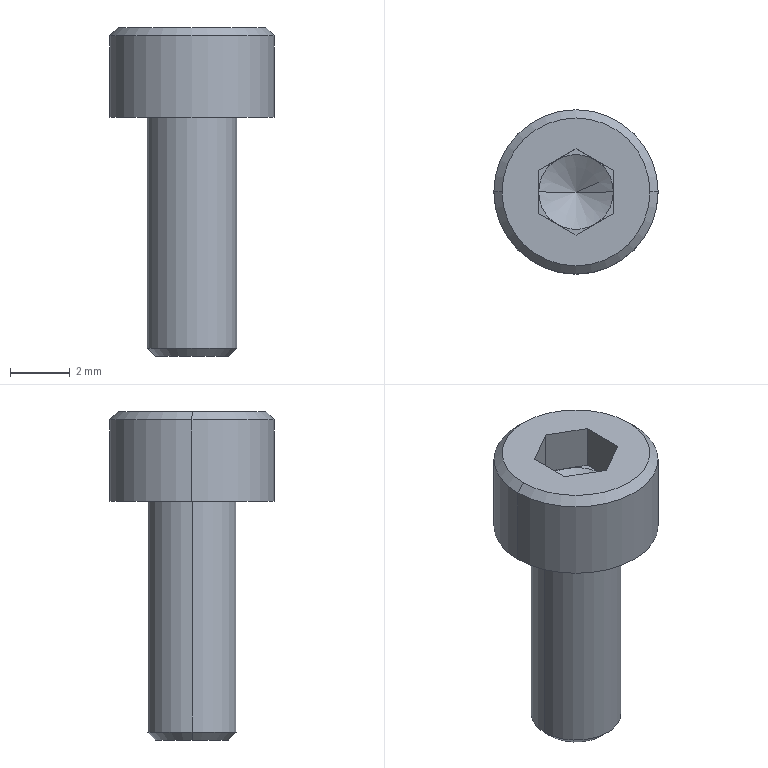Part | SolidWorks | features ICE 2, Chamfer 1, RevCut 1, Revolution 1 | 1 solid | 25 faces | box 5.5 x 5.5 x 11 mm | volume 117.558 mm3 | plane 15 | cone 6 | cylinder 4 | commonest cylinder face diameters 3 x2 5.5 x2
STEP:
#1=CARTESIAN_POINT('',(2.475,0.,3.));
#2=VERTEX_POINT('',#1);
#3=CARTESIAN_POINT('',(-2.475,0.,3.));
#4=VERTEX_POINT('',#3);
#5=CARTESIAN_POINT('',(0.,0.,3.));
#6=DIRECTION('',(0.,0.,1.));
#7=DIRECTION('',(1.,0.,0.));
#8=AXIS2_PLACEMENT_3D('',#5,#6,#7);
#9=CIRCLE('',#8,2.475);
#10=EDGE_CURVE('',#2,#4,#9,.T.);
#11=ORIENTED_EDGE('',*,*,#10,.F.);
#12=CARTESIAN_POINT('',(2.75,0.,2.725));
#13=VERTEX_POINT('',#12);
#14=CARTESIAN_POINT('',(2.475,0.,3.));
#15=DIRECTION('',(0.7071,0.,-0.7071));
#16=VECTOR('',#15,1000.);
#17=LINE('',#14,#16);
#18=EDGE_CURVE('',#2,#13,#17,.T.);
#19=ORIENTED_EDGE('',*,*,#18,.T.);
#20=CARTESIAN_POINT('',(-2.75,0.,2.725));
#21=VERTEX_POINT('',#20);
#22=CARTESIAN_POINT('',(0.,0.,2.725));
#23=DIRECTION('',(0.,0.,-1.));
#24=DIRECTION('',(1.,0.,0.));
#25=AXIS2_PLACEMENT_3D('',#22,#23,#24);
#26=CIRCLE('',#25,2.75);
#27=EDGE_CURVE('',#21,#13,#26,.T.);
#28=ORIENTED_EDGE('',*,*,#27,.F.);
#29=CARTESIAN_POINT('',(-2.475,0.,3.));
#30=DIRECTION('',(-0.7071,0.,-0.7071));
#31=VECTOR('',#30,1000.);
#32=LINE('',#29,#31);
#33=EDGE_CURVE('',#4,#21,#32,.T.);
#34=ORIENTED_EDGE('',*,*,#33,.F.);
#35=EDGE_LOOP('',(#11,#19,#28,#34));
#36=FACE_OUTER_BOUND('',#35,.T.);
#37=CARTESIAN_POINT('',(0.,0.,3.));
#38=DIRECTION('',(0.,0.,-1.));
#39=DIRECTION('',(-1.,0.,0.));
#40=AXIS2_PLACEMENT_3D('',#37,#38,#39);
#41=CONICAL_SURFACE('',#40,2.475,0.7854);
#42=ADVANCED_FACE('',(#36),#41,.T.);
#43=CARTESIAN_POINT('',(-1.225,0.,-8.));
#44=VERTEX_POINT('',#43);
#45=CARTESIAN_POINT('',(1.225,0.,-8.));
#46=VERTEX_POINT('',#45);
#47=CARTESIAN_POINT('',(0.,0.,-8.));
#48=DIRECTION('',(0.,0.,-1.));
#49=DIRECTION('',(-1.,0.,0.));
#50=AXIS2_PLACEMENT_3D('',#47,#48,#49);
#51=CIRCLE('',#50,1.225);
#52=EDGE_CURVE('',#44,#46,#51,.T.);
#53=ORIENTED_EDGE('',*,*,#52,.F.);
#54=CARTESIAN_POINT('',(-1.5,0.,-7.725));
#55=VERTEX_POINT('',#54);
#56=CARTESIAN_POINT('',(-1.225,0.,-8.));
#57=DIRECTION('',(-0.7071,0.,0.7071));
#58=VECTOR('',#57,1000.);
#59=LINE('',#56,#58);
#60=EDGE_CURVE('',#44,#55,#59,.T.);
#61=ORIENTED_EDGE('',*,*,#60,.T.);
#62=CARTESIAN_POINT('',(1.5,0.,-7.725));
#63=VERTEX_POINT('',#62);
#64=CARTESIAN_POINT('',(0.,0.,-7.725));
#65=DIRECTION('',(0.,0.,1.));
#66=DIRECTION('',(-1.,0.,0.));
#67=AXIS2_PLACEMENT_3D('',#64,#65,#66);
#68=CIRCLE('',#67,1.5);
#69=EDGE_CURVE('',#63,#55,#68,.T.);
#70=ORIENTED_EDGE('',*,*,#69,.F.);
#71=CARTESIAN_POINT('',(1.225,0.,-8.));
#72=DIRECTION('',(0.7071,0.,0.7071));
#73=VECTOR('',#72,1000.);
#74=LINE('',#71,#73);
#75=EDGE_CURVE('',#46,#63,#74,.T.);
#76=ORIENTED_EDGE('',*,*,#75,.F.);
#77=EDGE_LOOP('',(#53,#61,#70,#76));
#78=FACE_OUTER_BOUND('',#77,.T.);
#79=CARTESIAN_POINT('',(0.,0.,-8.));
#80=DIRECTION('',(0.,0.,1.));
#81=DIRECTION('',(1.,0.,0.));
#82=AXIS2_PLACEMENT_3D('',#79,#80,#81);
#83=CONICAL_SURFACE('',#82,1.225,0.7854);
#84=ADVANCED_FACE('',(#78),#83,.T.);
#85=CARTESIAN_POINT('',(0.,0.,0.7783));
#86=VERTEX_POINT('',#85);
#87=CARTESIAN_POINT('',(1.25,0.,1.5));
#88=VERTEX_POINT('',#87);
#89=CARTESIAN_POINT('',(0.,0.,0.7783));
#90=DIRECTION('',(0.866,0.,0.5));
#91=VECTOR('',#90,1000.);
#92=LINE('',#89,#91);
#93=EDGE_CURVE('',#86,#88,#92,.T.);
#94=ORIENTED_EDGE('',*,*,#93,.F.);
#95=CARTESIAN_POINT('',(-1.25,0.,1.5));
#96=VERTEX_POINT('',#95);
#97=CARTESIAN_POINT('',(0.,0.,0.7783));
#98=DIRECTION('',(-0.866,0.,0.5));
#99=VECTOR('',#98,1000.);
#100=LINE('',#97,#99);
#101=EDGE_CURVE('',#86,#96,#100,.T.);
#102=ORIENTED_EDGE('',*,*,#101,.T.);
#103=CARTESIAN_POINT('',(-0.625,-1.083,1.5));
#104=VERTEX_POINT('',#103);
#105=CARTESIAN_POINT('',(0.,0.,1.5));
#106=DIRECTION('',(0.,0.,-1.));
#107=DIRECTION('',(-1.,0.,0.));
#108=AXIS2_PLACEMENT_3D('',#105,#106,#107);
#109=CIRCLE('',#108,1.25);
#110=EDGE_CURVE('',#104,#96,#109,.T.);
#111=ORIENTED_EDGE('',*,*,#110,.F.);
#112=CARTESIAN_POINT('',(0.625,-1.083,1.5));
#113=VERTEX_POINT('',#112);
#114=CARTESIAN_POINT('',(0.,0.,1.5));
#115=DIRECTION('',(0.,0.,-1.));
#116=DIRECTION('',(-1.,0.,0.));
#117=AXIS2_PLACEMENT_3D('',#114,#115,#116);
#118=CIRCLE('',#117,1.25);
#119=EDGE_CURVE('',#113,#104,#118,.T.);
#120=ORIENTED_EDGE('',*,*,#119,.F.);
#121=CARTESIAN_POINT('',(0.,0.,1.5));
#122=DIRECTION('',(0.,0.,-1.));
#123=DIRECTION('',(-1.,0.,0.));
#124=AXIS2_PLACEMENT_3D('',#121,#122,#123);
#125=CIRCLE('',#124,1.25);
#126=EDGE_CURVE('',#88,#113,#125,.T.);
#127=ORIENTED_EDGE('',*,*,#126,.F.);
#128=EDGE_LOOP('',(#94,#102,#111,#120,#127));
#129=FACE_OUTER_BOUND('',#128,.T.);
#130=CARTESIAN_POINT('',(0.,0.,1000.778));
#131=DIRECTION('',(0.,0.,1.));
#132=DIRECTION('',(1.,0.,0.));
#133=AXIS2_PLACEMENT_3D('',#130,#131,#132);
#134=CONICAL_SURFACE('',#133,1732.051,1.047);
#135=ADVANCED_FACE('',(#129),#134,.F.);
#136=ORIENTED_EDGE('',*,*,#69,.T.);
#137=CARTESIAN_POINT('',(-1.5,0.,0.));
#138=VERTEX_POINT('',#137);
#139=CARTESIAN_POINT('',(-1.5,0.,-8.));
#140=DIRECTION('',(0.,0.,1.));
#141=VECTOR('',#140,1000.);
#142=LINE('',#139,#141);
#143=EDGE_CURVE('',#55,#138,#142,.T.);
#144=ORIENTED_EDGE('',*,*,#143,.T.);
#145=CARTESIAN_POINT('',(1.5,0.,0.));
#146=VERTEX_POINT('',#145);
#147=CARTESIAN_POINT('',(0.,0.,0.));
#148=DIRECTION('',(0.,0.,-1.));
#149=DIRECTION('',(-1.,0.,0.));
#150=AXIS2_PLACEMENT_3D('',#147,#148,#149);
#151=CIRCLE('',#150,1.5);
#152=EDGE_CURVE('',#138,#146,#151,.T.);
#153=ORIENTED_EDGE('',*,*,#152,.T.);
#154=CARTESIAN_POINT('',(1.5,0.,-8.));
#155=DIRECTION('',(0.,0.,1.));
#156=VECTOR('',#155,1000.);
#157=LINE('',#154,#156);
#158=EDGE_CURVE('',#63,#146,#157,.T.);
#159=ORIENTED_EDGE('',*,*,#158,.F.);
#160=EDGE_LOOP('',(#136,#144,#153,#159));
#161=FACE_OUTER_BOUND('',#160,.T.);
#162=CARTESIAN_POINT('',(0.,0.,-8.));
#163=DIRECTION('',(0.,0.,1.));
#164=DIRECTION('',(1.,0.,0.));
#165=AXIS2_PLACEMENT_3D('',#162,#163,#164);
#166=CYLINDRICAL_SURFACE('',#165,1.5);
#167=ADVANCED_FACE('',(#161),#166,.T.);
#168=CARTESIAN_POINT('',(2.75,0.,0.));
#169=VERTEX_POINT('',#168);
#170=CARTESIAN_POINT('',(-2.75,0.,0.));
#171=VERTEX_POINT('',#170);
#172=CARTESIAN_POINT('',(0.,0.,0.));
#173=DIRECTION('',(0.,0.,1.));
#174=DIRECTION('',(1.,0.,0.));
#175=AXIS2_PLACEMENT_3D('',#172,#173,#174);
#176=CIRCLE('',#175,2.75);
#177=EDGE_CURVE('',#169,#171,#176,.T.);
#178=ORIENTED_EDGE('',*,*,#177,.T.);
#179=CARTESIAN_POINT('',(-2.75,0.,0.));
#180=DIRECTION('',(0.,0.,1.));
#181=VECTOR('',#180,1000.);
#182=LINE('',#179,#181);
#183=EDGE_CURVE('',#171,#21,#182,.T.);
#184=ORIENTED_EDGE('',*,*,#183,.T.);
#185=ORIENTED_EDGE('',*,*,#27,.T.);
#186=CARTESIAN_POINT('',(2.75,0.,0.));
#187=DIRECTION('',(0.,0.,1.));
#188=VECTOR('',#187,1000.);
#189=LINE('',#186,#188);
#190=EDGE_CURVE('',#169,#13,#189,.T.);
#191=ORIENTED_EDGE('',*,*,#190,.F.);
#192=EDGE_LOOP('',(#178,#184,#185,#191));
#193=FACE_OUTER_BOUND('',#192,.T.);
#194=CARTESIAN_POINT('',(0.,0.,0.));
#195=DIRECTION('',(0.,0.,1.));
#196=DIRECTION('',(1.,0.,0.));
#197=AXIS2_PLACEMENT_3D('',#194,#195,#196);
#198=CYLINDRICAL_SURFACE('',#197,2.75);
#199=ADVANCED_FACE('',(#193),#198,.T.);
#200=CARTESIAN_POINT('',(-1.25,0.7217,1.5));
#201=VERTEX_POINT('',#200);
#202=CARTESIAN_POINT('',(-1.25,0.7217,1.5));
#203=DIRECTION('',(0.,-1.,0.));
#204=VECTOR('',#203,1000.);
#205=LINE('',#202,#204);
#206=EDGE_CURVE('',#201,#96,#205,.T.);
#207=ORIENTED_EDGE('',*,*,#206,.T.);
#208=CARTESIAN_POINT('',(-0.625,1.083,1.5));
#209=VERTEX_POINT('',#208);
#210=CARTESIAN_POINT('',(0.,0.,1.5));
#211=DIRECTION('',(0.,0.,-1.));
#212=DIRECTION('',(-1.,0.,0.));
#213=AXIS2_PLACEMENT_3D('',#210,#211,#212);
#214=CIRCLE('',#213,1.25);
#215=EDGE_CURVE('',#96,#209,#214,.T.);
#216=ORIENTED_EDGE('',*,*,#215,.T.);
#217=CARTESIAN_POINT('',(0.,1.443,1.5));
#218=DIRECTION('',(-0.866,-0.5,0.));
#219=VECTOR('',#218,1000.);
#220=LINE('',#217,#219);
#221=EDGE_CURVE('',#209,#201,#220,.T.);
#222=ORIENTED_EDGE('',*,*,#221,.T.);
#223=EDGE_LOOP('',(#207,#216,#222));
#224=FACE_OUTER_BOUND('',#223,.T.);
#225=CARTESIAN_POINT('',(0.,0.,1.5));
#226=DIRECTION('',(0.,0.,1.));
#227=DIRECTION('',(1.,0.,0.));
#228=AXIS2_PLACEMENT_3D('',#225,#226,#227);
#229=PLANE('',#228);
#230=ADVANCED_FACE('',(#224),#229,.T.);
#231=CARTESIAN_POINT('',(0.,1.443,1.5));
#232=VERTEX_POINT('',#231);
#233=CARTESIAN_POINT('',(0.,1.443,1.5));
#234=DIRECTION('',(-0.866,-0.5,0.));
#235=VECTOR('',#234,1000.);
#236=LINE('',#233,#235);
#237=EDGE_CURVE('',#232,#209,#236,.T.);
#238=ORIENTED_EDGE('',*,*,#237,.T.);
#239=CARTESIAN_POINT('',(0.625,1.083,1.5));
#240=VERTEX_POINT('',#239);
#241=CARTESIAN_POINT('',(0.,0.,1.5));
#242=DIRECTION('',(0.,0.,-1.));
#243=DIRECTION('',(-1.,0.,0.));
#244=AXIS2_PLACEMENT_3D('',#241,#242,#243);
#245=CIRCLE('',#244,1.25);
#246=EDGE_CURVE('',#209,#240,#245,.T.);
#247=ORIENTED_EDGE('',*,*,#246,.T.);
#248=CARTESIAN_POINT('',(1.25,0.7217,1.5));
#249=DIRECTION('',(-0.866,0.5,0.));
#250=VECTOR('',#249,1000.);
#251=LINE('',#248,#250);
#252=EDGE_CURVE('',#240,#232,#251,.T.);
#253=ORIENTED_EDGE('',*,*,#252,.T.);
#254=EDGE_LOOP('',(#238,#247,#253));
#255=FACE_OUTER_BOUND('',#254,.T.);
#256=CARTESIAN_POINT('',(0.,0.,1.5));
#257=DIRECTION('',(0.,0.,1.));
#258=DIRECTION('',(1.,0.,0.));
#259=AXIS2_PLACEMENT_3D('',#256,#257,#258);
#260=PLANE('',#259);
#261=ADVANCED_FACE('',(#255),#260,.T.);
#262=CARTESIAN_POINT('',(1.25,0.7217,1.5));
#263=VERTEX_POINT('',#262);
#264=CARTESIAN_POINT('',(1.25,0.7217,1.5));
#265=DIRECTION('',(-0.866,0.5,0.));
#266=VECTOR('',#265,1000.);
#267=LINE('',#264,#266);
#268=EDGE_CURVE('',#263,#240,#267,.T.);
#269=ORIENTED_EDGE('',*,*,#268,.T.);
#270=CARTESIAN_POINT('',(0.,0.,1.5));
#271=DIRECTION('',(0.,0.,-1.));
#272=DIRECTION('',(-1.,0.,0.));
#273=AXIS2_PLACEMENT_3D('',#270,#271,#272);
#274=CIRCLE('',#273,1.25);
#275=EDGE_CURVE('',#240,#88,#274,.T.);
#276=ORIENTED_EDGE('',*,*,#275,.T.);
#277=CARTESIAN_POINT('',(1.25,-0.7217,1.5));
#278=DIRECTION('',(0.,1.,0.));
#279=VECTOR('',#278,1000.);
#280=LINE('',#277,#279);
#281=EDGE_CURVE('',#88,#263,#280,.T.);
#282=ORIENTED_EDGE('',*,*,#281,.T.);
#283=EDGE_LOOP('',(#269,#276,#282));
#284=FACE_OUTER_BOUND('',#283,.T.);
#285=CARTESIAN_POINT('',(0.,0.,1.5));
#286=DIRECTION('',(0.,0.,1.));
#287=DIRECTION('',(1.,0.,0.));
#288=AXIS2_PLACEMENT_3D('',#285,#286,#287);
#289=PLANE('',#288);
#290=ADVANCED_FACE('',(#284),#289,.T.);
#291=CARTESIAN_POINT('',(1.25,-0.7217,1.5));
#292=VERTEX_POINT('',#291);
#293=CARTESIAN_POINT('',(1.25,-0.7217,1.5));
#294=DIRECTION('',(0.,1.,0.));
#295=VECTOR('',#294,1000.);
#296=LINE('',#293,#295);
#297=EDGE_CURVE('',#292,#88,#296,.T.);
#298=ORIENTED_EDGE('',*,*,#297,.T.);
#299=ORIENTED_EDGE('',*,*,#126,.T.);
#300=CARTESIAN_POINT('',(0.,-1.443,1.5));
#301=DIRECTION('',(0.866,0.5,0.));
#302=VECTOR('',#301,1000.);
#303=LINE('',#300,#302);
#304=EDGE_CURVE('',#113,#292,#303,.T.);
#305=ORIENTED_EDGE('',*,*,#304,.T.);
#306=EDGE_LOOP('',(#298,#299,#305));
#307=FACE_OUTER_BOUND('',#306,.T.);
#308=CARTESIAN_POINT('',(0.,0.,1.5));
#309=DIRECTION('',(0.,0.,1.));
#310=DIRECTION('',(1.,0.,0.));
#311=AXIS2_PLACEMENT_3D('',#308,#309,#310);
#312=PLANE('',#311);
#313=ADVANCED_FACE('',(#307),#312,.T.);
#314=CARTESIAN_POINT('',(0.,-1.443,1.5));
#315=VERTEX_POINT('',#314);
#316=CARTESIAN_POINT('',(0.,-1.443,1.5));
#317=DIRECTION('',(0.866,0.5,0.));
#318=VECTOR('',#317,1000.);
#319=LINE('',#316,#318);
#320=EDGE_CURVE('',#315,#113,#319,.T.);
#321=ORIENTED_EDGE('',*,*,#320,.T.);
#322=ORIENTED_EDGE('',*,*,#119,.T.);
#323=CARTESIAN_POINT('',(-1.25,-0.7217,1.5));
#324=DIRECTION('',(0.866,-0.5,0.));
#325=VECTOR('',#324,1000.);
#326=LINE('',#323,#325);
#327=EDGE_CURVE('',#104,#315,#326,.T.);
#328=ORIENTED_EDGE('',*,*,#327,.T.);
#329=EDGE_LOOP('',(#321,#322,#328));
#330=FACE_OUTER_BOUND('',#329,.T.);
#331=CARTESIAN_POINT('',(0.,0.,1.5));
#332=DIRECTION('',(0.,0.,1.));
#333=DIRECTION('',(1.,0.,0.));
#334=AXIS2_PLACEMENT_3D('',#331,#332,#333);
#335=PLANE('',#334);
#336=ADVANCED_FACE('',(#330),#335,.T.);
#337=CARTESIAN_POINT('',(-1.25,-0.7217,1.5));
#338=VERTEX_POINT('',#337);
#339=CARTESIAN_POINT('',(-1.25,-0.7217,1.5));
#340=DIRECTION('',(0.866,-0.5,0.));
#341=VECTOR('',#340,1000.);
#342=LINE('',#339,#341);
#343=EDGE_CURVE('',#338,#104,#342,.T.);
#344=ORIENTED_EDGE('',*,*,#343,.T.);
#345=ORIENTED_EDGE('',*,*,#110,.T.);
#346=CARTESIAN_POINT('',(-1.25,0.7217,1.5));
#347=DIRECTION('',(0.,-1.,0.));
#348=VECTOR('',#347,1000.);
#349=LINE('',#346,#348);
#350=EDGE_CURVE('',#96,#338,#349,.T.);
#351=ORIENTED_EDGE('',*,*,#350,.T.);
#352=EDGE_LOOP('',(#344,#345,#351));
#353=FACE_OUTER_BOUND('',#352,.T.);
#354=CARTESIAN_POINT('',(0.,0.,1.5));
#355=DIRECTION('',(0.,0.,1.));
#356=DIRECTION('',(1.,0.,0.));
#357=AXIS2_PLACEMENT_3D('',#354,#355,#356);
#358=PLANE('',#357);
#359=ADVANCED_FACE('',(#353),#358,.T.);
#360=ORIENTED_EDGE('',*,*,#177,.F.);
#361=CARTESIAN_POINT('',(0.,0.,0.));
#362=DIRECTION('',(0.,0.,1.));
#363=DIRECTION('',(1.,0.,0.));
#364=AXIS2_PLACEMENT_3D('',#361,#362,#363);
#365=CIRCLE('',#364,2.75);
#366=EDGE_CURVE('',#171,#169,#365,.T.);
#367=ORIENTED_EDGE('',*,*,#366,.F.);
#368=EDGE_LOOP('',(#360,#367));
#369=FACE_OUTER_BOUND('',#368,.T.);
#370=CARTESIAN_POINT('',(0.,0.,0.));
#371=DIRECTION('',(0.,0.,-1.));
#372=DIRECTION('',(-1.,0.,0.));
#373=AXIS2_PLACEMENT_3D('',#370,#371,#372);
#374=CIRCLE('',#373,1.5);
#375=EDGE_CURVE('',#146,#138,#374,.T.);
#376=ORIENTED_EDGE('',*,*,#375,.F.);
#377=ORIENTED_EDGE('',*,*,#152,.F.);
#378=EDGE_LOOP('',(#376,#377));
#379=FACE_BOUND('',#378,.T.);
#380=CARTESIAN_POINT('',(2.75,0.,0.));
#381=DIRECTION('',(0.,0.,-1.));
#382=DIRECTION('',(-1.,0.,0.));
#383=AXIS2_PLACEMENT_3D('',#380,#381,#382);
#384=PLANE('',#383);
#385=ADVANCED_FACE('',(#369,#379),#384,.T.);
#386=ORIENTED_EDGE('',*,*,#183,.F.);
#387=ORIENTED_EDGE('',*,*,#366,.T.);
#388=ORIENTED_EDGE('',*,*,#190,.T.);
#389=CARTESIAN_POINT('',(0.,0.,2.725));
#390=DIRECTION('',(0.,0.,-1.));
#391=DIRECTION('',(1.,0.,0.));
#392=AXIS2_PLACEMENT_3D('',#389,#390,#391);
#393=CIRCLE('',#392,2.75);
#394=EDGE_CURVE('',#13,#21,#393,.T.);
#395=ORIENTED_EDGE('',*,*,#394,.T.);
#396=EDGE_LOOP('',(#386,#387,#388,#395));
#397=FACE_OUTER_BOUND('',#396,.T.);
#398=CARTESIAN_POINT('',(0.,0.,0.));
#399=DIRECTION('',(0.,0.,1.));
#400=DIRECTION('',(1.,0.,0.));
#401=AXIS2_PLACEMENT_3D('',#398,#399,#400);
#402=CYLINDRICAL_SURFACE('',#401,2.75);
#403=ADVANCED_FACE('',(#397),#402,.T.);
#404=CARTESIAN_POINT('',(0.,0.,3.));
#405=DIRECTION('',(0.,0.,1.));
#406=DIRECTION('',(1.,0.,0.));
#407=AXIS2_PLACEMENT_3D('',#404,#405,#406);
#408=CIRCLE('',#407,2.475);
#409=EDGE_CURVE('',#4,#2,#408,.T.);
#410=ORIENTED_EDGE('',*,*,#409,.T.);
#411=ORIENTED_EDGE('',*,*,#10,.T.);
#412=EDGE_LOOP('',(#410,#411));
#413=FACE_OUTER_BOUND('',#412,.T.);
#414=CARTESIAN_POINT('',(0.,-1.443,3.));
#415=VERTEX_POINT('',#414);
#416=CARTESIAN_POINT('',(1.25,-0.7217,3.));
#417=VERTEX_POINT('',#416);
#418=CARTESIAN_POINT('',(0.,-1.443,3.));
#419=DIRECTION('',(0.866,0.5,0.));
#420=VECTOR('',#419,1000.);
#421=LINE('',#418,#420);
#422=EDGE_CURVE('',#415,#417,#421,.T.);
#423=ORIENTED_EDGE('',*,*,#422,.F.);
#424=CARTESIAN_POINT('',(-1.25,-0.7217,3.));
#425=VERTEX_POINT('',#424);
#426=CARTESIAN_POINT('',(-1.25,-0.7217,3.));
#427=DIRECTION('',(0.866,-0.5,0.));
#428=VECTOR('',#427,1000.);
#429=LINE('',#426,#428);
#430=EDGE_CURVE('',#425,#415,#429,.T.);
#431=ORIENTED_EDGE('',*,*,#430,.F.);
#432=CARTESIAN_POINT('',(-1.25,0.7217,3.));
#433=VERTEX_POINT('',#432);
#434=CARTESIAN_POINT('',(-1.25,0.7217,3.));
#435=DIRECTION('',(0.,-1.,0.));
#436=VECTOR('',#435,1000.);
#437=LINE('',#434,#436);
#438=EDGE_CURVE('',#433,#425,#437,.T.);
#439=ORIENTED_EDGE('',*,*,#438,.F.);
#440=CARTESIAN_POINT('',(0.,1.443,3.));
#441=VERTEX_POINT('',#440);
#442=CARTESIAN_POINT('',(0.,1.443,3.));
#443=DIRECTION('',(-0.866,-0.5,0.));
#444=VECTOR('',#443,1000.);
#445=LINE('',#442,#444);
#446=EDGE_CURVE('',#441,#433,#445,.T.);
#447=ORIENTED_EDGE('',*,*,#446,.F.);
#448=CARTESIAN_POINT('',(1.25,0.7217,3.));
#449=VERTEX_POINT('',#448);
#450=CARTESIAN_POINT('',(1.25,0.7217,3.));
#451=DIRECTION('',(-0.866,0.5,0.));
#452=VECTOR('',#451,1000.);
#453=LINE('',#450,#452);
#454=EDGE_CURVE('',#449,#441,#453,.T.);
#455=ORIENTED_EDGE('',*,*,#454,.F.);
#456=CARTESIAN_POINT('',(1.25,-0.7217,3.));
#457=DIRECTION('',(0.,1.,0.));
#458=VECTOR('',#457,1000.);
#459=LINE('',#456,#458);
#460=EDGE_CURVE('',#417,#449,#459,.T.);
#461=ORIENTED_EDGE('',*,*,#460,.F.);
#462=EDGE_LOOP('',(#423,#431,#439,#447,#455,#461));
#463=FACE_BOUND('',#462,.T.);
#464=CARTESIAN_POINT('',(0.,0.,3.));
#465=DIRECTION('',(0.,0.,1.));
#466=DIRECTION('',(1.,0.,0.));
#467=AXIS2_PLACEMENT_3D('',#464,#465,#466);
#468=PLANE('',#467);
#469=ADVANCED_FACE('',(#413,#463),#468,.T.);
#470=ORIENTED_EDGE('',*,*,#143,.F.);
#471=CARTESIAN_POINT('',(0.,0.,-7.725));
#472=DIRECTION('',(0.,0.,1.));
#473=DIRECTION('',(-1.,0.,0.));
#474=AXIS2_PLACEMENT_3D('',#471,#472,#473);
#475=CIRCLE('',#474,1.5);
#476=EDGE_CURVE('',#55,#63,#475,.T.);
#477=ORIENTED_EDGE('',*,*,#476,.T.);
#478=ORIENTED_EDGE('',*,*,#158,.T.);
#479=ORIENTED_EDGE('',*,*,#375,.T.);
#480=EDGE_LOOP('',(#470,#477,#478,#479));
#481=FACE_OUTER_BOUND('',#480,.T.);
#482=CARTESIAN_POINT('',(0.,0.,-8.));
#483=DIRECTION('',(0.,0.,1.));
#484=DIRECTION('',(1.,0.,0.));
#485=AXIS2_PLACEMENT_3D('',#482,#483,#484);
#486=CYLINDRICAL_SURFACE('',#485,1.5);
#487=ADVANCED_FACE('',(#481),#486,.T.);
#488=CARTESIAN_POINT('',(0.,0.,-8.));
#489=DIRECTION('',(0.,0.,-1.));
#490=DIRECTION('',(-1.,0.,0.));
#491=AXIS2_PLACEMENT_3D('',#488,#489,#490);
#492=CIRCLE('',#491,1.225);
#493=EDGE_CURVE('',#46,#44,#492,.T.);
#494=ORIENTED_EDGE('',*,*,#493,.T.);
#495=ORIENTED_EDGE('',*,*,#52,.T.);
#496=EDGE_LOOP('',(#494,#495));
#497=FACE_OUTER_BOUND('',#496,.T.);
#498=CARTESIAN_POINT('',(0.,0.,-8.));
#499=DIRECTION('',(0.,0.,-1.));
#500=DIRECTION('',(-1.,0.,0.));
#501=AXIS2_PLACEMENT_3D('',#498,#499,#500);
#502=PLANE('',#501);
#503=ADVANCED_FACE('',(#497),#502,.T.);
#504=ORIENTED_EDGE('',*,*,#422,.T.);
#505=CARTESIAN_POINT('',(1.25,-0.7217,1.5));
#506=DIRECTION('',(0.,0.,1.));
#507=VECTOR('',#506,1000.);
#508=LINE('',#505,#507);
#509=EDGE_CURVE('',#292,#417,#508,.T.);
#510=ORIENTED_EDGE('',*,*,#509,.F.);
#511=ORIENTED_EDGE('',*,*,#304,.F.);
#512=ORIENTED_EDGE('',*,*,#320,.F.);
#513=CARTESIAN_POINT('',(0.,-1.443,1.5));
#514=DIRECTION('',(0.,0.,1.));
#515=VECTOR('',#514,1000.);
#516=LINE('',#513,#515);
#517=EDGE_CURVE('',#315,#415,#516,.T.);
#518=ORIENTED_EDGE('',*,*,#517,.T.);
#519=EDGE_LOOP('',(#504,#510,#511,#512,#518));
#520=FACE_OUTER_BOUND('',#519,.T.);
#521=CARTESIAN_POINT('',(0.,-1.443,1.5));
#522=DIRECTION('',(0.5,-0.866,0.));
#523=DIRECTION('',(0.866,0.5,0.));
#524=AXIS2_PLACEMENT_3D('',#521,#522,#523);
#525=PLANE('',#524);
#526=ADVANCED_FACE('',(#520),#525,.F.);
#527=ORIENTED_EDGE('',*,*,#430,.T.);
#528=ORIENTED_EDGE('',*,*,#517,.F.);
#529=ORIENTED_EDGE('',*,*,#327,.F.);
#530=ORIENTED_EDGE('',*,*,#343,.F.);
#531=CARTESIAN_POINT('',(-1.25,-0.7217,1.5));
#532=DIRECTION('',(0.,0.,1.));
#533=VECTOR('',#532,1000.);
#534=LINE('',#531,#533);
#535=EDGE_CURVE('',#338,#425,#534,.T.);
#536=ORIENTED_EDGE('',*,*,#535,.T.);
#537=EDGE_LOOP('',(#527,#528,#529,#530,#536));
#538=FACE_OUTER_BOUND('',#537,.T.);
#539=CARTESIAN_POINT('',(-1.25,-0.7217,1.5));
#540=DIRECTION('',(-0.5,-0.866,0.));
#541=DIRECTION('',(0.866,-0.5,0.));
#542=AXIS2_PLACEMENT_3D('',#539,#540,#541);
#543=PLANE('',#542);
#544=ADVANCED_FACE('',(#538),#543,.F.);
#545=ORIENTED_EDGE('',*,*,#438,.T.);
#546=ORIENTED_EDGE('',*,*,#535,.F.);
#547=ORIENTED_EDGE('',*,*,#350,.F.);
#548=ORIENTED_EDGE('',*,*,#206,.F.);
#549=CARTESIAN_POINT('',(-1.25,0.7217,1.5));
#550=DIRECTION('',(0.,0.,1.));
#551=VECTOR('',#550,1000.);
#552=LINE('',#549,#551);
#553=EDGE_CURVE('',#201,#433,#552,.T.);
#554=ORIENTED_EDGE('',*,*,#553,.T.);
#555=EDGE_LOOP('',(#545,#546,#547,#548,#554));
#556=FACE_OUTER_BOUND('',#555,.T.);
#557=CARTESIAN_POINT('',(-1.25,0.7217,1.5));
#558=DIRECTION('',(-1.,0.,0.));
#559=DIRECTION('',(0.,-1.,0.));
#560=AXIS2_PLACEMENT_3D('',#557,#558,#559);
#561=PLANE('',#560);
#562=ADVANCED_FACE('',(#556),#561,.F.);
#563=ORIENTED_EDGE('',*,*,#446,.T.);
#564=ORIENTED_EDGE('',*,*,#553,.F.);
#565=ORIENTED_EDGE('',*,*,#221,.F.);
#566=ORIENTED_EDGE('',*,*,#237,.F.);
#567=CARTESIAN_POINT('',(0.,1.443,1.5));
#568=DIRECTION('',(0.,0.,1.));
#569=VECTOR('',#568,1000.);
#570=LINE('',#567,#569);
#571=EDGE_CURVE('',#232,#441,#570,.T.);
#572=ORIENTED_EDGE('',*,*,#571,.T.);
#573=EDGE_LOOP('',(#563,#564,#565,#566,#572));
#574=FACE_OUTER_BOUND('',#573,.T.);
#575=CARTESIAN_POINT('',(0.,1.443,1.5));
#576=DIRECTION('',(-0.5,0.866,0.));
#577=DIRECTION('',(-0.866,-0.5,0.));
#578=AXIS2_PLACEMENT_3D('',#575,#576,#577);
#579=PLANE('',#578);
#580=ADVANCED_FACE('',(#574),#579,.F.);
#581=ORIENTED_EDGE('',*,*,#454,.T.);
#582=ORIENTED_EDGE('',*,*,#571,.F.);
#583=ORIENTED_EDGE('',*,*,#252,.F.);
#584=ORIENTED_EDGE('',*,*,#268,.F.);
#585=CARTESIAN_POINT('',(1.25,0.7217,1.5));
#586=DIRECTION('',(0.,0.,1.));
#587=VECTOR('',#586,1000.);
#588=LINE('',#585,#587);
#589=EDGE_CURVE('',#263,#449,#588,.T.);
#590=ORIENTED_EDGE('',*,*,#589,.T.);
#591=EDGE_LOOP('',(#581,#582,#583,#584,#590));
#592=FACE_OUTER_BOUND('',#591,.T.);
#593=CARTESIAN_POINT('',(1.25,0.7217,1.5));
#594=DIRECTION('',(0.5,0.866,0.));
#595=DIRECTION('',(-0.866,0.5,0.));
#596=AXIS2_PLACEMENT_3D('',#593,#594,#595);
#597=PLANE('',#596);
#598=ADVANCED_FACE('',(#592),#597,.F.);
#599=ORIENTED_EDGE('',*,*,#460,.T.);
#600=ORIENTED_EDGE('',*,*,#589,.F.);
#601=ORIENTED_EDGE('',*,*,#281,.F.);
#602=ORIENTED_EDGE('',*,*,#297,.F.);
#603=ORIENTED_EDGE('',*,*,#509,.T.);
#604=EDGE_LOOP('',(#599,#600,#601,#602,#603));
#605=FACE_OUTER_BOUND('',#604,.T.);
#606=CARTESIAN_POINT('',(1.25,-0.7217,1.5));
#607=DIRECTION('',(1.,0.,0.));
#608=DIRECTION('',(0.,0.,-1.));
#609=AXIS2_PLACEMENT_3D('',#606,#607,#608);
#610=PLANE('',#609);
#611=ADVANCED_FACE('',(#605),#610,.F.);
#612=ORIENTED_EDGE('',*,*,#101,.F.);
#613=ORIENTED_EDGE('',*,*,#93,.T.);
#614=ORIENTED_EDGE('',*,*,#275,.F.);
#615=ORIENTED_EDGE('',*,*,#246,.F.);
#616=ORIENTED_EDGE('',*,*,#215,.F.);
#617=EDGE_LOOP('',(#612,#613,#614,#615,#616));
#618=FACE_OUTER_BOUND('',#617,.T.);
#619=CARTESIAN_POINT('',(0.,0.,1000.778));
#620=DIRECTION('',(0.,0.,1.));
#621=DIRECTION('',(1.,0.,0.));
#622=AXIS2_PLACEMENT_3D('',#619,#620,#621);
#623=CONICAL_SURFACE('',#622,1732.051,1.047);
#624=ADVANCED_FACE('',(#618),#623,.F.);
#625=ORIENTED_EDGE('',*,*,#60,.F.);
#626=ORIENTED_EDGE('',*,*,#493,.F.);
#627=ORIENTED_EDGE('',*,*,#75,.T.);
#628=ORIENTED_EDGE('',*,*,#476,.F.);
#629=EDGE_LOOP('',(#625,#626,#627,#628));
#630=FACE_OUTER_BOUND('',#629,.T.);
#631=CARTESIAN_POINT('',(0.,0.,-8.));
#632=DIRECTION('',(0.,0.,1.));
#633=DIRECTION('',(1.,0.,0.));
#634=AXIS2_PLACEMENT_3D('',#631,#632,#633);
#635=CONICAL_SURFACE('',#634,1.225,0.7854);
#636=ADVANCED_FACE('',(#630),#635,.T.);
#637=ORIENTED_EDGE('',*,*,#18,.F.);
#638=ORIENTED_EDGE('',*,*,#409,.F.);
#639=ORIENTED_EDGE('',*,*,#33,.T.);
#640=ORIENTED_EDGE('',*,*,#394,.F.);
#641=EDGE_LOOP('',(#637,#638,#639,#640));
#642=FACE_OUTER_BOUND('',#641,.T.);
#643=CARTESIAN_POINT('',(0.,0.,3.));
#644=DIRECTION('',(0.,0.,-1.));
#645=DIRECTION('',(-1.,0.,0.));
#646=AXIS2_PLACEMENT_3D('',#643,#644,#645);
#647=CONICAL_SURFACE('',#646,2.475,0.7854);
#648=ADVANCED_FACE('',(#642),#647,.T.);
#649=CLOSED_SHELL('',(#42,#84,#135,#167,#199,#230,#261,#290,#313,#336,#359,#385,#403,#469,#487,#503,#526,#544,#562,#580,#598,#611,#624,#636,#648));
#650=MANIFOLD_SOLID_BREP('',#649);
#651=CARTESIAN_POINT('',(0.,0.,0.));
#652=DIRECTION('',(0.,0.,1.));
#653=DIRECTION('',(1.,0.,0.));
#654=AXIS2_PLACEMENT_3D('',#651,#652,#653);
#655=(LENGTH_UNIT()NAMED_UNIT(*)SI_UNIT(.MILLI.,.METRE.));
#656=UNCERTAINTY_MEASURE_WITH_UNIT(LENGTH_MEASURE(0.00001),#655,'','');
#657=(NAMED_UNIT(*)PLANE_ANGLE_UNIT()SI_UNIT($,.RADIAN.));
#658=(NAMED_UNIT(*)SI_UNIT($,.STERADIAN.)SOLID_ANGLE_UNIT());
#659=(GEOMETRIC_REPRESENTATION_CONTEXT(3)GLOBAL_UNCERTAINTY_ASSIGNED_CONTEXT((#656))GLOBAL_UNIT_ASSIGNED_CONTEXT((#655,#657,#658))REPRESENTATION_CONTEXT('',''));
#660=ADVANCED_BREP_SHAPE_REPRESENTATION('',(#650,#654),#659);